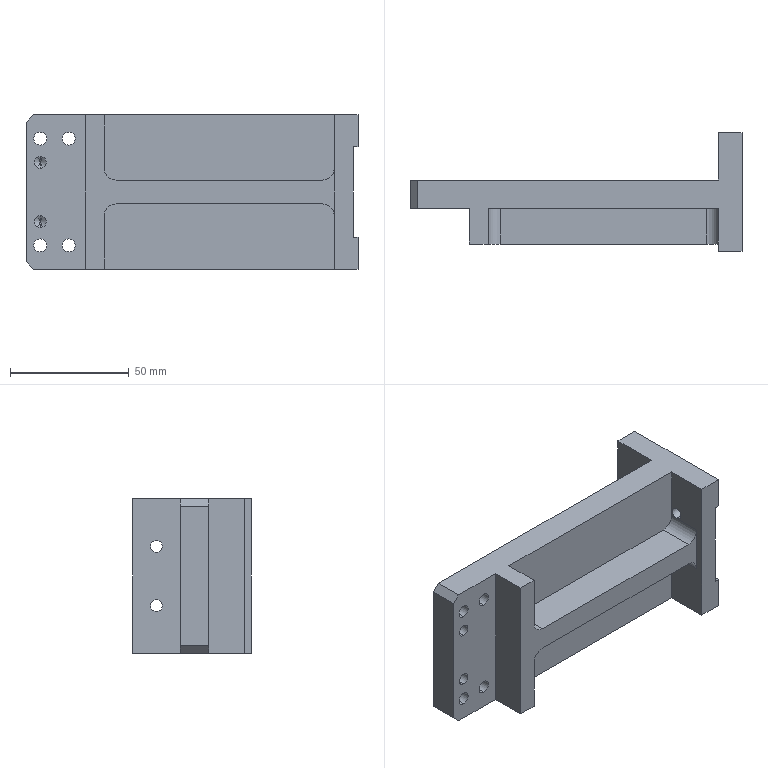Part | NX | features BREP 1 | 1 solid | 64 faces | box 140 x 50 x 65 mm | volume 149431 mm3 | cylinder 32 | plane 28 | cone 4 | commonest cylinder face diameters 5 x12 5.5 x8 9.999 x8 10 x4